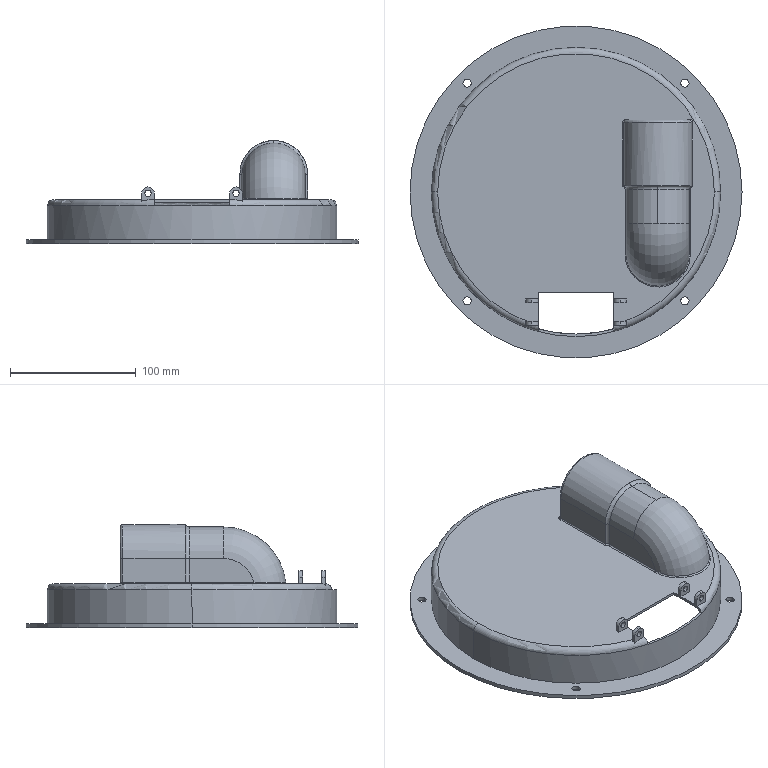Part | SolidWorks | features Fillet 6, ICE 6, Sweep 2, CirPattern 1, CombineBodies 1, Cut 1, Extrusion 1, MirrorPattern 1, Shell 1 | 1 solid | 90 faces | box 264 x 264 x 82 mm | volume 198550 mm3 | cylinder 45 | plane 27 | torus 16 | spline 2 | commonest cylinder face diameters 5 x8 6.5 x8 10 x8 2 x4 6 x4 4 x2